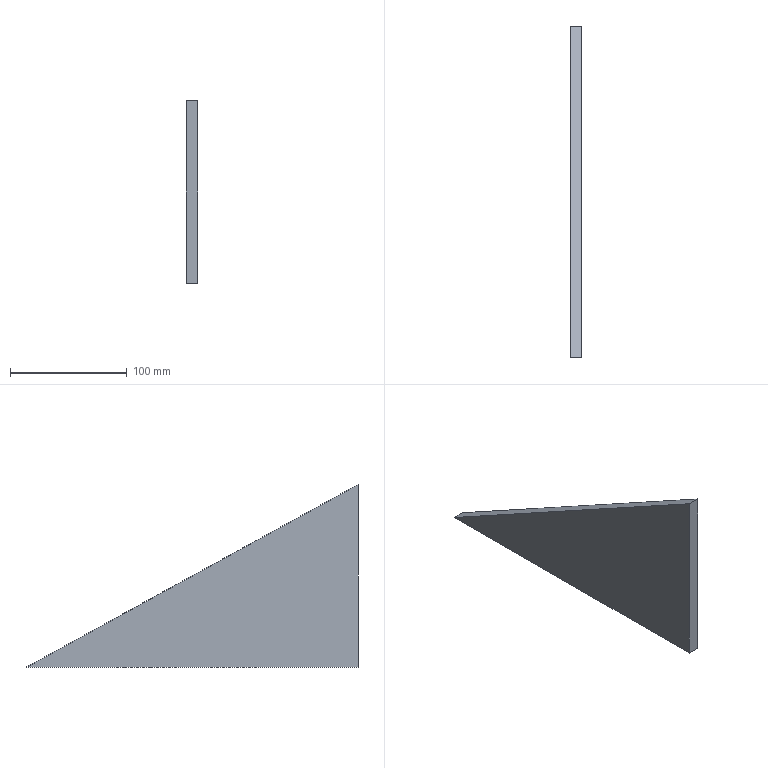Part | STEP file | 1 solid | 5 faces | box 10 x 283.933 x 156.359 mm | volume 221977 mm3 | plane 5
STEP:
#1=CARTESIAN_POINT('',(0.,0.,0.));
#2=DIRECTION('',(0.,0.,1.));
#3=DIRECTION('',(1.,0.,0.));
#4=AXIS2_PLACEMENT_3D('',#1,#2,#3);
#5=CARTESIAN_POINT('',(-533.841,103.097,-50.));
#6=VERTEX_POINT('',#5);
#7=CARTESIAN_POINT('',(-533.841,-180.836,-50.));
#8=VERTEX_POINT('',#7);
#9=CARTESIAN_POINT('',(-533.841,-180.836,-50.));
#10=DIRECTION('',(0.,-1.,0.));
#11=VECTOR('',#10,1.);
#12=LINE('',#9,#11);
#13=CARTESIAN_POINT('',(-543.841,-180.836,-50.));
#14=DIRECTION('',(0.,0.,1.));
#15=DIRECTION('',(1.,0.,0.));
#16=AXIS2_PLACEMENT_3D('',#13,#14,#15);
#17=PLANE('',#16);
#18=CARTESIAN_POINT('',(10.,0.));
#19=DIRECTION('',(0.,-1.));
#20=VECTOR('',#19,1.);
#21=LINE('',#18,#20);
#22=(GEOMETRIC_REPRESENTATION_CONTEXT(2)PARAMETRIC_REPRESENTATION_CONTEXT()REPRESENTATION_CONTEXT('',''));
#23=DEFINITIONAL_REPRESENTATION('',(#21),#22);
#24=PCURVE('',#17,#23);
#25=CARTESIAN_POINT('',(-533.841,0.,0.));
#26=DIRECTION('',(-1.,0.,0.));
#27=DIRECTION('',(0.,0.,1.));
#28=AXIS2_PLACEMENT_3D('',#25,#26,#27);
#29=PLANE('',#28);
#30=CARTESIAN_POINT('',(-50.,-180.836));
#31=DIRECTION('',(0.,-1.));
#32=VECTOR('',#31,1.);
#33=LINE('',#30,#32);
#34=(GEOMETRIC_REPRESENTATION_CONTEXT(2)PARAMETRIC_REPRESENTATION_CONTEXT()REPRESENTATION_CONTEXT('',''));
#35=DEFINITIONAL_REPRESENTATION('',(#33),#34);
#36=PCURVE('',#29,#35);
#37=SURFACE_CURVE('',#12,(#24,#36),.PCURVE_S1.);
#38=EDGE_CURVE('',#6,#8,#37,.T.);
#39=ORIENTED_EDGE('',*,*,#38,.T.);
#40=CARTESIAN_POINT('',(-543.841,-180.836,-50.));
#41=VERTEX_POINT('',#40);
#42=CARTESIAN_POINT('',(-543.841,-180.836,-50.));
#43=DIRECTION('',(1.,0.,0.));
#44=VECTOR('',#43,1.);
#45=LINE('',#42,#44);
#46=CARTESIAN_POINT('',(0.,0.));
#47=DIRECTION('',(1.,0.));
#48=VECTOR('',#47,1.);
#49=LINE('',#46,#48);
#50=(GEOMETRIC_REPRESENTATION_CONTEXT(2)PARAMETRIC_REPRESENTATION_CONTEXT()REPRESENTATION_CONTEXT('',''));
#51=DEFINITIONAL_REPRESENTATION('',(#49),#50);
#52=PCURVE('',#17,#51);
#53=CARTESIAN_POINT('',(-543.841,-180.836,106.359));
#54=DIRECTION('',(0.,1.,0.));
#55=DIRECTION('',(0.,0.,1.));
#56=AXIS2_PLACEMENT_3D('',#53,#54,#55);
#57=PLANE('',#56);
#58=CARTESIAN_POINT('',(-156.359,0.));
#59=DIRECTION('',(0.,1.));
#60=VECTOR('',#59,1.);
#61=LINE('',#58,#60);
#62=(GEOMETRIC_REPRESENTATION_CONTEXT(2)PARAMETRIC_REPRESENTATION_CONTEXT()REPRESENTATION_CONTEXT('',''));
#63=DEFINITIONAL_REPRESENTATION('',(#61),#62);
#64=PCURVE('',#57,#63);
#65=SURFACE_CURVE('',#45,(#52,#64),.PCURVE_S1.);
#66=EDGE_CURVE('',#41,#8,#65,.T.);
#67=ORIENTED_EDGE('',*,*,#66,.F.);
#68=CARTESIAN_POINT('',(-543.841,103.097,-50.));
#69=VERTEX_POINT('',#68);
#70=CARTESIAN_POINT('',(-543.841,-180.836,-50.));
#71=DIRECTION('',(0.,-1.,0.));
#72=VECTOR('',#71,1.);
#73=LINE('',#70,#72);
#74=CARTESIAN_POINT('',(0.,0.));
#75=DIRECTION('',(0.,-1.));
#76=VECTOR('',#75,1.);
#77=LINE('',#74,#76);
#78=(GEOMETRIC_REPRESENTATION_CONTEXT(2)PARAMETRIC_REPRESENTATION_CONTEXT()REPRESENTATION_CONTEXT('',''));
#79=DEFINITIONAL_REPRESENTATION('',(#77),#78);
#80=PCURVE('',#17,#79);
#81=CARTESIAN_POINT('',(-543.841,0.,0.));
#82=DIRECTION('',(-1.,0.,0.));
#83=DIRECTION('',(0.,0.,1.));
#84=AXIS2_PLACEMENT_3D('',#81,#82,#83);
#85=PLANE('',#84);
#86=CARTESIAN_POINT('',(-50.,-180.836));
#87=DIRECTION('',(0.,-1.));
#88=VECTOR('',#87,1.);
#89=LINE('',#86,#88);
#90=(GEOMETRIC_REPRESENTATION_CONTEXT(2)PARAMETRIC_REPRESENTATION_CONTEXT()REPRESENTATION_CONTEXT('',''));
#91=DEFINITIONAL_REPRESENTATION('',(#89),#90);
#92=PCURVE('',#85,#91);
#93=SURFACE_CURVE('',#73,(#80,#92),.PCURVE_S1.);
#94=EDGE_CURVE('',#69,#41,#93,.T.);
#95=ORIENTED_EDGE('',*,*,#94,.F.);
#96=CARTESIAN_POINT('',(-543.841,103.097,-50.));
#97=DIRECTION('',(1.,0.,0.));
#98=VECTOR('',#97,1.);
#99=LINE('',#96,#98);
#100=CARTESIAN_POINT('',(0.,283.933));
#101=DIRECTION('',(1.,0.));
#102=VECTOR('',#101,1.);
#103=LINE('',#100,#102);
#104=(GEOMETRIC_REPRESENTATION_CONTEXT(2)PARAMETRIC_REPRESENTATION_CONTEXT()REPRESENTATION_CONTEXT('',''));
#105=DEFINITIONAL_REPRESENTATION('',(#103),#104);
#106=PCURVE('',#17,#105);
#107=CARTESIAN_POINT('',(-543.841,103.097,-50.));
#108=DIRECTION('',(0.,-0.4824,-0.876));
#109=DIRECTION('',(0.,0.876,-0.4824));
#110=AXIS2_PLACEMENT_3D('',#107,#108,#109);
#111=PLANE('',#110);
#112=CARTESIAN_POINT('',(0.,0.));
#113=DIRECTION('',(0.,1.));
#114=VECTOR('',#113,1.);
#115=LINE('',#112,#114);
#116=(GEOMETRIC_REPRESENTATION_CONTEXT(2)PARAMETRIC_REPRESENTATION_CONTEXT()REPRESENTATION_CONTEXT('',''));
#117=DEFINITIONAL_REPRESENTATION('',(#115),#116);
#118=PCURVE('',#111,#117);
#119=SURFACE_CURVE('',#99,(#106,#118),.PCURVE_S1.);
#120=EDGE_CURVE('',#69,#6,#119,.T.);
#121=ORIENTED_EDGE('',*,*,#120,.T.);
#122=EDGE_LOOP('',(#39,#67,#95,#121));
#123=FACE_BOUND('',#122,.T.);
#124=ADVANCED_FACE('',(#123),#17,.F.);
#125=CARTESIAN_POINT('',(-533.841,-180.836,106.359));
#126=VERTEX_POINT('',#125);
#127=CARTESIAN_POINT('',(-533.841,-180.836,106.359));
#128=DIRECTION('',(0.,0.,1.));
#129=VECTOR('',#128,1.);
#130=LINE('',#127,#129);
#131=CARTESIAN_POINT('',(0.,10.));
#132=DIRECTION('',(1.,0.));
#133=VECTOR('',#132,1.);
#134=LINE('',#131,#133);
#135=(GEOMETRIC_REPRESENTATION_CONTEXT(2)PARAMETRIC_REPRESENTATION_CONTEXT()REPRESENTATION_CONTEXT('',''));
#136=DEFINITIONAL_REPRESENTATION('',(#134),#135);
#137=PCURVE('',#57,#136);
#138=CARTESIAN_POINT('',(106.359,-180.836));
#139=DIRECTION('',(1.,0.));
#140=VECTOR('',#139,1.);
#141=LINE('',#138,#140);
#142=(GEOMETRIC_REPRESENTATION_CONTEXT(2)PARAMETRIC_REPRESENTATION_CONTEXT()REPRESENTATION_CONTEXT('',''));
#143=DEFINITIONAL_REPRESENTATION('',(#141),#142);
#144=PCURVE('',#29,#143);
#145=SURFACE_CURVE('',#130,(#137,#144),.PCURVE_S1.);
#146=EDGE_CURVE('',#8,#126,#145,.T.);
#147=ORIENTED_EDGE('',*,*,#146,.T.);
#148=CARTESIAN_POINT('',(-543.841,-180.836,106.359));
#149=VERTEX_POINT('',#148);
#150=CARTESIAN_POINT('',(-543.841,-180.836,106.359));
#151=DIRECTION('',(1.,0.,0.));
#152=VECTOR('',#151,1.);
#153=LINE('',#150,#152);
#154=CARTESIAN_POINT('',(0.,0.));
#155=DIRECTION('',(0.,1.));
#156=VECTOR('',#155,1.);
#157=LINE('',#154,#156);
#158=(GEOMETRIC_REPRESENTATION_CONTEXT(2)PARAMETRIC_REPRESENTATION_CONTEXT()REPRESENTATION_CONTEXT('',''));
#159=DEFINITIONAL_REPRESENTATION('',(#157),#158);
#160=PCURVE('',#57,#159);
#161=CARTESIAN_POINT('',(-324.139,0.));
#162=DIRECTION('',(0.,1.));
#163=VECTOR('',#162,1.);
#164=LINE('',#161,#163);
#165=(GEOMETRIC_REPRESENTATION_CONTEXT(2)PARAMETRIC_REPRESENTATION_CONTEXT()REPRESENTATION_CONTEXT('',''));
#166=DEFINITIONAL_REPRESENTATION('',(#164),#165);
#167=PCURVE('',#111,#166);
#168=SURFACE_CURVE('',#153,(#160,#167),.PCURVE_S1.);
#169=EDGE_CURVE('',#149,#126,#168,.T.);
#170=ORIENTED_EDGE('',*,*,#169,.F.);
#171=CARTESIAN_POINT('',(-543.841,-180.836,106.359));
#172=DIRECTION('',(0.,0.,1.));
#173=VECTOR('',#172,1.);
#174=LINE('',#171,#173);
#175=CARTESIAN_POINT('',(0.,0.));
#176=DIRECTION('',(1.,0.));
#177=VECTOR('',#176,1.);
#178=LINE('',#175,#177);
#179=(GEOMETRIC_REPRESENTATION_CONTEXT(2)PARAMETRIC_REPRESENTATION_CONTEXT()REPRESENTATION_CONTEXT('',''));
#180=DEFINITIONAL_REPRESENTATION('',(#178),#179);
#181=PCURVE('',#57,#180);
#182=CARTESIAN_POINT('',(106.359,-180.836));
#183=DIRECTION('',(1.,0.));
#184=VECTOR('',#183,1.);
#185=LINE('',#182,#184);
#186=(GEOMETRIC_REPRESENTATION_CONTEXT(2)PARAMETRIC_REPRESENTATION_CONTEXT()REPRESENTATION_CONTEXT('',''));
#187=DEFINITIONAL_REPRESENTATION('',(#185),#186);
#188=PCURVE('',#85,#187);
#189=SURFACE_CURVE('',#174,(#181,#188),.PCURVE_S1.);
#190=EDGE_CURVE('',#41,#149,#189,.T.);
#191=ORIENTED_EDGE('',*,*,#190,.F.);
#192=ORIENTED_EDGE('',*,*,#66,.T.);
#193=EDGE_LOOP('',(#147,#170,#191,#192));
#194=FACE_BOUND('',#193,.T.);
#195=ADVANCED_FACE('',(#194),#57,.F.);
#196=CARTESIAN_POINT('',(-533.841,103.097,-50.));
#197=DIRECTION('',(0.,0.876,-0.4824));
#198=VECTOR('',#197,1.);
#199=LINE('',#196,#198);
#200=CARTESIAN_POINT('',(0.,10.));
#201=DIRECTION('',(1.,0.));
#202=VECTOR('',#201,1.);
#203=LINE('',#200,#202);
#204=(GEOMETRIC_REPRESENTATION_CONTEXT(2)PARAMETRIC_REPRESENTATION_CONTEXT()REPRESENTATION_CONTEXT('',''));
#205=DEFINITIONAL_REPRESENTATION('',(#203),#204);
#206=PCURVE('',#111,#205);
#207=CARTESIAN_POINT('',(-50.,103.097));
#208=DIRECTION('',(-0.4824,0.876));
#209=VECTOR('',#208,1.);
#210=LINE('',#207,#209);
#211=(GEOMETRIC_REPRESENTATION_CONTEXT(2)PARAMETRIC_REPRESENTATION_CONTEXT()REPRESENTATION_CONTEXT('',''));
#212=DEFINITIONAL_REPRESENTATION('',(#210),#211);
#213=PCURVE('',#29,#212);
#214=SURFACE_CURVE('',#199,(#206,#213),.PCURVE_S1.);
#215=EDGE_CURVE('',#126,#6,#214,.T.);
#216=ORIENTED_EDGE('',*,*,#215,.T.);
#217=ORIENTED_EDGE('',*,*,#120,.F.);
#218=CARTESIAN_POINT('',(-543.841,103.097,-50.));
#219=DIRECTION('',(0.,0.876,-0.4824));
#220=VECTOR('',#219,1.);
#221=LINE('',#218,#220);
#222=CARTESIAN_POINT('',(0.,0.));
#223=DIRECTION('',(1.,0.));
#224=VECTOR('',#223,1.);
#225=LINE('',#222,#224);
#226=(GEOMETRIC_REPRESENTATION_CONTEXT(2)PARAMETRIC_REPRESENTATION_CONTEXT()REPRESENTATION_CONTEXT('',''));
#227=DEFINITIONAL_REPRESENTATION('',(#225),#226);
#228=PCURVE('',#111,#227);
#229=CARTESIAN_POINT('',(-50.,103.097));
#230=DIRECTION('',(-0.4824,0.876));
#231=VECTOR('',#230,1.);
#232=LINE('',#229,#231);
#233=(GEOMETRIC_REPRESENTATION_CONTEXT(2)PARAMETRIC_REPRESENTATION_CONTEXT()REPRESENTATION_CONTEXT('',''));
#234=DEFINITIONAL_REPRESENTATION('',(#232),#233);
#235=PCURVE('',#85,#234);
#236=SURFACE_CURVE('',#221,(#228,#235),.PCURVE_S1.);
#237=EDGE_CURVE('',#149,#69,#236,.T.);
#238=ORIENTED_EDGE('',*,*,#237,.F.);
#239=ORIENTED_EDGE('',*,*,#169,.T.);
#240=EDGE_LOOP('',(#216,#217,#238,#239));
#241=FACE_BOUND('',#240,.T.);
#242=ADVANCED_FACE('',(#241),#111,.F.);
#243=ORIENTED_EDGE('',*,*,#94,.T.);
#244=ORIENTED_EDGE('',*,*,#190,.T.);
#245=ORIENTED_EDGE('',*,*,#237,.T.);
#246=EDGE_LOOP('',(#243,#244,#245));
#247=FACE_BOUND('',#246,.T.);
#248=ADVANCED_FACE('',(#247),#85,.T.);
#249=ORIENTED_EDGE('',*,*,#38,.F.);
#250=ORIENTED_EDGE('',*,*,#215,.F.);
#251=ORIENTED_EDGE('',*,*,#146,.F.);
#252=EDGE_LOOP('',(#249,#250,#251));
#253=FACE_BOUND('',#252,.T.);
#254=ADVANCED_FACE('',(#253),#29,.F.);
#255=CLOSED_SHELL('',(#124,#195,#242,#248,#254));
#256=MANIFOLD_SOLID_BREP('',#255);
#257=(LENGTH_UNIT()NAMED_UNIT(*)SI_UNIT(.MILLI.,.METRE.));
#258=UNCERTAINTY_MEASURE_WITH_UNIT(LENGTH_MEASURE(0.0000001),#257,'','');
#259=(NAMED_UNIT(*)PLANE_ANGLE_UNIT()SI_UNIT($,.RADIAN.));
#260=(NAMED_UNIT(*)SI_UNIT($,.STERADIAN.)SOLID_ANGLE_UNIT());
#261=(GEOMETRIC_REPRESENTATION_CONTEXT(3)GLOBAL_UNCERTAINTY_ASSIGNED_CONTEXT((#258))GLOBAL_UNIT_ASSIGNED_CONTEXT((#257,#259,#260))REPRESENTATION_CONTEXT('',''));
#262=ADVANCED_BREP_SHAPE_REPRESENTATION('',(#4,#256),#261);